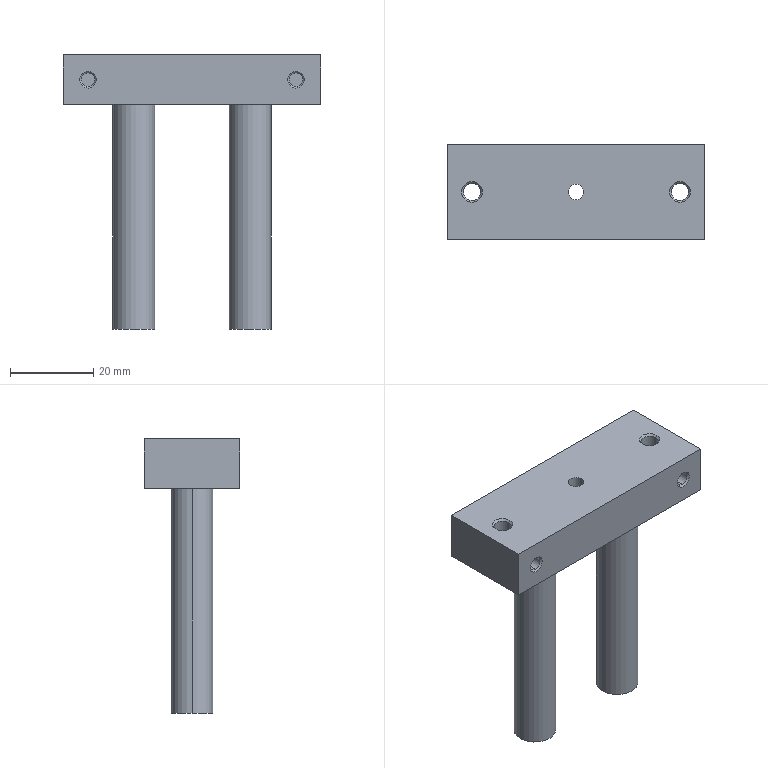Part | STEP file | rod_A_CXSM20_40_Z80_0_ | 1 solid | 42 faces | box 62 x 23 x 66 mm | volume 24938 mm3 | cylinder 18 | cone 12 | plane 12 | commonest cylinder face diameters 3.24 x8 4.13 x4 10 x4 3.732 x2
STEP:
#1=CARTESIAN_POINT('',(-1.866,12.5,12.));
#2=VERTEX_POINT('',#1);
#3=CARTESIAN_POINT('',(1.866,12.5,12.));
#4=VERTEX_POINT('',#3);
#5=CARTESIAN_POINT('',(0.,12.5,12.));
#6=DIRECTION('',(0.,0.,1.));
#7=DIRECTION('',(1.,0.,0.));
#8=AXIS2_PLACEMENT_3D('',#5,#6,#7);
#9=CIRCLE('',#8,1.866);
#10=EDGE_CURVE('',#2,#4,#9,.T.);
#11=ORIENTED_EDGE('',*,*,#10,.F.);
#12=CARTESIAN_POINT('',(-1.866,12.5,24.));
#13=VERTEX_POINT('',#12);
#14=CARTESIAN_POINT('',(-1.866,12.5,-42.));
#15=DIRECTION('',(0.,0.,1.));
#16=VECTOR('',#15,1000.);
#17=LINE('',#14,#16);
#18=EDGE_CURVE('',#2,#13,#17,.T.);
#19=ORIENTED_EDGE('',*,*,#18,.T.);
#20=CARTESIAN_POINT('',(1.866,12.5,24.));
#21=VERTEX_POINT('',#20);
#22=CARTESIAN_POINT('',(0.,12.5,24.));
#23=DIRECTION('',(0.,0.,1.));
#24=DIRECTION('',(1.,0.,0.));
#25=AXIS2_PLACEMENT_3D('',#22,#23,#24);
#26=CIRCLE('',#25,1.866);
#27=EDGE_CURVE('',#13,#21,#26,.T.);
#28=ORIENTED_EDGE('',*,*,#27,.T.);
#29=CARTESIAN_POINT('',(1.866,12.5,-42.));
#30=DIRECTION('',(0.,0.,1.));
#31=VECTOR('',#30,1000.);
#32=LINE('',#29,#31);
#33=EDGE_CURVE('',#4,#21,#32,.T.);
#34=ORIENTED_EDGE('',*,*,#33,.F.);
#35=EDGE_LOOP('',(#11,#19,#28,#34));
#36=FACE_OUTER_BOUND('',#35,.T.);
#37=CARTESIAN_POINT('',(0.,12.5,-42.));
#38=DIRECTION('',(0.,0.,1.));
#39=DIRECTION('',(1.,0.,0.));
#40=AXIS2_PLACEMENT_3D('',#37,#38,#39);
#41=CYLINDRICAL_SURFACE('',#40,1.866);
#42=ADVANCED_FACE('',(#36),#41,.F.);
#43=CARTESIAN_POINT('',(-25.,1.38,16.38));
#44=VERTEX_POINT('',#43);
#45=CARTESIAN_POINT('',(-25.,1.38,19.62));
#46=VERTEX_POINT('',#45);
#47=CARTESIAN_POINT('',(-25.,1.38,18.));
#48=DIRECTION('',(0.,1.,0.));
#49=DIRECTION('',(0.,0.,1.));
#50=AXIS2_PLACEMENT_3D('',#47,#48,#49);
#51=CIRCLE('',#50,1.62);
#52=EDGE_CURVE('',#44,#46,#51,.T.);
#53=ORIENTED_EDGE('',*,*,#52,.F.);
#54=CARTESIAN_POINT('',(-25.,7.,16.38));
#55=VERTEX_POINT('',#54);
#56=CARTESIAN_POINT('',(-25.,0.,16.38));
#57=DIRECTION('',(0.,1.,0.));
#58=VECTOR('',#57,1000.);
#59=LINE('',#56,#58);
#60=EDGE_CURVE('',#44,#55,#59,.T.);
#61=ORIENTED_EDGE('',*,*,#60,.T.);
#62=CARTESIAN_POINT('',(-25.,7.,19.62));
#63=VERTEX_POINT('',#62);
#64=CARTESIAN_POINT('',(-25.,7.,18.));
#65=DIRECTION('',(0.,1.,0.));
#66=DIRECTION('',(0.,0.,1.));
#67=AXIS2_PLACEMENT_3D('',#64,#65,#66);
#68=CIRCLE('',#67,1.62);
#69=EDGE_CURVE('',#55,#63,#68,.T.);
#70=ORIENTED_EDGE('',*,*,#69,.T.);
#71=CARTESIAN_POINT('',(-25.,0.,19.62));
#72=DIRECTION('',(0.,1.,0.));
#73=VECTOR('',#72,1000.);
#74=LINE('',#71,#73);
#75=EDGE_CURVE('',#46,#63,#74,.T.);
#76=ORIENTED_EDGE('',*,*,#75,.F.);
#77=EDGE_LOOP('',(#53,#61,#70,#76));
#78=FACE_OUTER_BOUND('',#77,.T.);
#79=CARTESIAN_POINT('',(-25.,0.,18.));
#80=DIRECTION('',(0.,1.,0.));
#81=DIRECTION('',(0.,0.,1.));
#82=AXIS2_PLACEMENT_3D('',#79,#80,#81);
#83=CYLINDRICAL_SURFACE('',#82,1.62);
#84=ADVANCED_FACE('',(#78),#83,.F.);
#85=ORIENTED_EDGE('',*,*,#52,.T.);
#86=CARTESIAN_POINT('',(-25.,1.,20.));
#87=VERTEX_POINT('',#86);
#88=CARTESIAN_POINT('',(-25.,0.,21.));
#89=DIRECTION('',(0.,-0.7071,0.7071));
#90=VECTOR('',#89,1000.);
#91=LINE('',#88,#90);
#92=EDGE_CURVE('',#46,#87,#91,.T.);
#93=ORIENTED_EDGE('',*,*,#92,.T.);
#94=CARTESIAN_POINT('',(-25.,1.,16.));
#95=VERTEX_POINT('',#94);
#96=CARTESIAN_POINT('',(-25.,1.,18.));
#97=DIRECTION('',(0.,-1.,0.));
#98=DIRECTION('',(0.,0.,1.));
#99=AXIS2_PLACEMENT_3D('',#96,#97,#98);
#100=CIRCLE('',#99,2.);
#101=EDGE_CURVE('',#87,#95,#100,.T.);
#102=ORIENTED_EDGE('',*,*,#101,.T.);
#103=CARTESIAN_POINT('',(-25.,0.,15.));
#104=DIRECTION('',(0.,-0.7071,-0.7071));
#105=VECTOR('',#104,1000.);
#106=LINE('',#103,#105);
#107=EDGE_CURVE('',#44,#95,#106,.T.);
#108=ORIENTED_EDGE('',*,*,#107,.F.);
#109=EDGE_LOOP('',(#85,#93,#102,#108));
#110=FACE_OUTER_BOUND('',#109,.T.);
#111=CARTESIAN_POINT('',(-25.,0.,18.));
#112=DIRECTION('',(0.,-1.,0.));
#113=DIRECTION('',(0.,0.,-1.));
#114=AXIS2_PLACEMENT_3D('',#111,#112,#113);
#115=CONICAL_SURFACE('',#114,3.,0.7854);
#116=ADVANCED_FACE('',(#110),#115,.F.);
#117=CARTESIAN_POINT('',(25.,1.38,16.38));
#118=VERTEX_POINT('',#117);
#119=CARTESIAN_POINT('',(25.,1.38,19.62));
#120=VERTEX_POINT('',#119);
#121=CARTESIAN_POINT('',(25.,1.38,18.));
#122=DIRECTION('',(0.,1.,0.));
#123=DIRECTION('',(0.,0.,1.));
#124=AXIS2_PLACEMENT_3D('',#121,#122,#123);
#125=CIRCLE('',#124,1.62);
#126=EDGE_CURVE('',#118,#120,#125,.T.);
#127=ORIENTED_EDGE('',*,*,#126,.F.);
#128=CARTESIAN_POINT('',(25.,7.,16.38));
#129=VERTEX_POINT('',#128);
#130=CARTESIAN_POINT('',(25.,0.,16.38));
#131=DIRECTION('',(0.,1.,0.));
#132=VECTOR('',#131,1000.);
#133=LINE('',#130,#132);
#134=EDGE_CURVE('',#118,#129,#133,.T.);
#135=ORIENTED_EDGE('',*,*,#134,.T.);
#136=CARTESIAN_POINT('',(25.,7.,19.62));
#137=VERTEX_POINT('',#136);
#138=CARTESIAN_POINT('',(25.,7.,18.));
#139=DIRECTION('',(0.,1.,0.));
#140=DIRECTION('',(0.,0.,1.));
#141=AXIS2_PLACEMENT_3D('',#138,#139,#140);
#142=CIRCLE('',#141,1.62);
#143=EDGE_CURVE('',#129,#137,#142,.T.);
#144=ORIENTED_EDGE('',*,*,#143,.T.);
#145=CARTESIAN_POINT('',(25.,0.,19.62));
#146=DIRECTION('',(0.,1.,0.));
#147=VECTOR('',#146,1000.);
#148=LINE('',#145,#147);
#149=EDGE_CURVE('',#120,#137,#148,.T.);
#150=ORIENTED_EDGE('',*,*,#149,.F.);
#151=EDGE_LOOP('',(#127,#135,#144,#150));
#152=FACE_OUTER_BOUND('',#151,.T.);
#153=CARTESIAN_POINT('',(25.,0.,18.));
#154=DIRECTION('',(0.,1.,0.));
#155=DIRECTION('',(0.,0.,1.));
#156=AXIS2_PLACEMENT_3D('',#153,#154,#155);
#157=CYLINDRICAL_SURFACE('',#156,1.62);
#158=ADVANCED_FACE('',(#152),#157,.F.);
#159=ORIENTED_EDGE('',*,*,#126,.T.);
#160=CARTESIAN_POINT('',(25.,1.,20.));
#161=VERTEX_POINT('',#160);
#162=CARTESIAN_POINT('',(25.,0.,21.));
#163=DIRECTION('',(0.,-0.7071,0.7071));
#164=VECTOR('',#163,1000.);
#165=LINE('',#162,#164);
#166=EDGE_CURVE('',#120,#161,#165,.T.);
#167=ORIENTED_EDGE('',*,*,#166,.T.);
#168=CARTESIAN_POINT('',(25.,1.,16.));
#169=VERTEX_POINT('',#168);
#170=CARTESIAN_POINT('',(25.,1.,18.));
#171=DIRECTION('',(0.,-1.,0.));
#172=DIRECTION('',(0.,0.,1.));
#173=AXIS2_PLACEMENT_3D('',#170,#171,#172);
#174=CIRCLE('',#173,2.);
#175=EDGE_CURVE('',#161,#169,#174,.T.);
#176=ORIENTED_EDGE('',*,*,#175,.T.);
#177=CARTESIAN_POINT('',(25.,0.,15.));
#178=DIRECTION('',(0.,-0.7071,-0.7071));
#179=VECTOR('',#178,1000.);
#180=LINE('',#177,#179);
#181=EDGE_CURVE('',#118,#169,#180,.T.);
#182=ORIENTED_EDGE('',*,*,#181,.F.);
#183=EDGE_LOOP('',(#159,#167,#176,#182));
#184=FACE_OUTER_BOUND('',#183,.T.);
#185=CARTESIAN_POINT('',(25.,0.,18.));
#186=DIRECTION('',(0.,-1.,0.));
#187=DIRECTION('',(0.,0.,-1.));
#188=AXIS2_PLACEMENT_3D('',#185,#186,#187);
#189=CONICAL_SURFACE('',#188,3.,0.7854);
#190=ADVANCED_FACE('',(#184),#189,.F.);
#191=CARTESIAN_POINT('',(-22.935,12.5,23.565));
#192=VERTEX_POINT('',#191);
#193=CARTESIAN_POINT('',(-27.065,12.5,23.565));
#194=VERTEX_POINT('',#193);
#195=CARTESIAN_POINT('',(-25.,12.5,23.565));
#196=DIRECTION('',(0.,0.,-1.));
#197=DIRECTION('',(-1.,0.,0.));
#198=AXIS2_PLACEMENT_3D('',#195,#196,#197);
#199=CIRCLE('',#198,2.065);
#200=EDGE_CURVE('',#192,#194,#199,.T.);
#201=ORIENTED_EDGE('',*,*,#200,.T.);
#202=CARTESIAN_POINT('',(-27.5,12.5,24.));
#203=VERTEX_POINT('',#202);
#204=CARTESIAN_POINT('',(-28.,12.5,24.5));
#205=DIRECTION('',(-0.7071,0.,0.7071));
#206=VECTOR('',#205,1000.);
#207=LINE('',#204,#206);
#208=EDGE_CURVE('',#194,#203,#207,.T.);
#209=ORIENTED_EDGE('',*,*,#208,.T.);
#210=CARTESIAN_POINT('',(-22.5,12.5,24.));
#211=VERTEX_POINT('',#210);
#212=CARTESIAN_POINT('',(-25.,12.5,24.));
#213=DIRECTION('',(0.,0.,-1.));
#214=DIRECTION('',(1.,0.,0.));
#215=AXIS2_PLACEMENT_3D('',#212,#213,#214);
#216=CIRCLE('',#215,2.5);
#217=EDGE_CURVE('',#211,#203,#216,.T.);
#218=ORIENTED_EDGE('',*,*,#217,.F.);
#219=CARTESIAN_POINT('',(-22.,12.5,24.5));
#220=DIRECTION('',(0.7071,0.,0.7071));
#221=VECTOR('',#220,1000.);
#222=LINE('',#219,#221);
#223=EDGE_CURVE('',#192,#211,#222,.T.);
#224=ORIENTED_EDGE('',*,*,#223,.F.);
#225=EDGE_LOOP('',(#201,#209,#218,#224));
#226=FACE_OUTER_BOUND('',#225,.T.);
#227=CARTESIAN_POINT('',(-25.,12.5,24.5));
#228=DIRECTION('',(0.,0.,1.));
#229=DIRECTION('',(1.,0.,0.));
#230=AXIS2_PLACEMENT_3D('',#227,#228,#229);
#231=CONICAL_SURFACE('',#230,3.,0.7854);
#232=ADVANCED_FACE('',(#226),#231,.F.);
#233=ORIENTED_EDGE('',*,*,#200,.F.);
#234=CARTESIAN_POINT('',(-22.935,12.5,12.));
#235=VERTEX_POINT('',#234);
#236=CARTESIAN_POINT('',(-22.935,12.5,24.5));
#237=DIRECTION('',(0.,0.,-1.));
#238=VECTOR('',#237,1000.);
#239=LINE('',#236,#238);
#240=EDGE_CURVE('',#192,#235,#239,.T.);
#241=ORIENTED_EDGE('',*,*,#240,.T.);
#242=CARTESIAN_POINT('',(-27.065,12.5,12.));
#243=VERTEX_POINT('',#242);
#244=CARTESIAN_POINT('',(-25.,12.5,12.));
#245=DIRECTION('',(0.,0.,-1.));
#246=DIRECTION('',(-1.,0.,0.));
#247=AXIS2_PLACEMENT_3D('',#244,#245,#246);
#248=CIRCLE('',#247,2.065);
#249=EDGE_CURVE('',#235,#243,#248,.T.);
#250=ORIENTED_EDGE('',*,*,#249,.T.);
#251=CARTESIAN_POINT('',(-27.065,12.5,24.5));
#252=DIRECTION('',(0.,0.,-1.));
#253=VECTOR('',#252,1000.);
#254=LINE('',#251,#253);
#255=EDGE_CURVE('',#194,#243,#254,.T.);
#256=ORIENTED_EDGE('',*,*,#255,.F.);
#257=EDGE_LOOP('',(#233,#241,#250,#256));
#258=FACE_OUTER_BOUND('',#257,.T.);
#259=CARTESIAN_POINT('',(-25.,12.5,24.5));
#260=DIRECTION('',(0.,0.,-1.));
#261=DIRECTION('',(-1.,0.,0.));
#262=AXIS2_PLACEMENT_3D('',#259,#260,#261);
#263=CYLINDRICAL_SURFACE('',#262,2.065);
#264=ADVANCED_FACE('',(#258),#263,.F.);
#265=CARTESIAN_POINT('',(27.065,12.5,23.565));
#266=VERTEX_POINT('',#265);
#267=CARTESIAN_POINT('',(22.935,12.5,23.565));
#268=VERTEX_POINT('',#267);
#269=CARTESIAN_POINT('',(25.,12.5,23.565));
#270=DIRECTION('',(0.,0.,-1.));
#271=DIRECTION('',(-1.,0.,0.));
#272=AXIS2_PLACEMENT_3D('',#269,#270,#271);
#273=CIRCLE('',#272,2.065);
#274=EDGE_CURVE('',#266,#268,#273,.T.);
#275=ORIENTED_EDGE('',*,*,#274,.T.);
#276=CARTESIAN_POINT('',(22.5,12.5,24.));
#277=VERTEX_POINT('',#276);
#278=CARTESIAN_POINT('',(22.,12.5,24.5));
#279=DIRECTION('',(-0.7071,0.,0.7071));
#280=VECTOR('',#279,1000.);
#281=LINE('',#278,#280);
#282=EDGE_CURVE('',#268,#277,#281,.T.);
#283=ORIENTED_EDGE('',*,*,#282,.T.);
#284=CARTESIAN_POINT('',(27.5,12.5,24.));
#285=VERTEX_POINT('',#284);
#286=CARTESIAN_POINT('',(25.,12.5,24.));
#287=DIRECTION('',(0.,0.,-1.));
#288=DIRECTION('',(1.,0.,0.));
#289=AXIS2_PLACEMENT_3D('',#286,#287,#288);
#290=CIRCLE('',#289,2.5);
#291=EDGE_CURVE('',#285,#277,#290,.T.);
#292=ORIENTED_EDGE('',*,*,#291,.F.);
#293=CARTESIAN_POINT('',(28.,12.5,24.5));
#294=DIRECTION('',(0.7071,0.,0.7071));
#295=VECTOR('',#294,1000.);
#296=LINE('',#293,#295);
#297=EDGE_CURVE('',#266,#285,#296,.T.);
#298=ORIENTED_EDGE('',*,*,#297,.F.);
#299=EDGE_LOOP('',(#275,#283,#292,#298));
#300=FACE_OUTER_BOUND('',#299,.T.);
#301=CARTESIAN_POINT('',(25.,12.5,24.5));
#302=DIRECTION('',(0.,0.,1.));
#303=DIRECTION('',(1.,0.,0.));
#304=AXIS2_PLACEMENT_3D('',#301,#302,#303);
#305=CONICAL_SURFACE('',#304,3.,0.7854);
#306=ADVANCED_FACE('',(#300),#305,.F.);
#307=ORIENTED_EDGE('',*,*,#274,.F.);
#308=CARTESIAN_POINT('',(27.065,12.5,12.));
#309=VERTEX_POINT('',#308);
#310=CARTESIAN_POINT('',(27.065,12.5,24.5));
#311=DIRECTION('',(0.,0.,-1.));
#312=VECTOR('',#311,1000.);
#313=LINE('',#310,#312);
#314=EDGE_CURVE('',#266,#309,#313,.T.);
#315=ORIENTED_EDGE('',*,*,#314,.T.);
#316=CARTESIAN_POINT('',(22.935,12.5,12.));
#317=VERTEX_POINT('',#316);
#318=CARTESIAN_POINT('',(25.,12.5,12.));
#319=DIRECTION('',(0.,0.,-1.));
#320=DIRECTION('',(-1.,0.,0.));
#321=AXIS2_PLACEMENT_3D('',#318,#319,#320);
#322=CIRCLE('',#321,2.065);
#323=EDGE_CURVE('',#309,#317,#322,.T.);
#324=ORIENTED_EDGE('',*,*,#323,.T.);
#325=CARTESIAN_POINT('',(22.935,12.5,24.5));
#326=DIRECTION('',(0.,0.,-1.));
#327=VECTOR('',#326,1000.);
#328=LINE('',#325,#327);
#329=EDGE_CURVE('',#268,#317,#328,.T.);
#330=ORIENTED_EDGE('',*,*,#329,.F.);
#331=EDGE_LOOP('',(#307,#315,#324,#330));
#332=FACE_OUTER_BOUND('',#331,.T.);
#333=CARTESIAN_POINT('',(25.,12.5,24.5));
#334=DIRECTION('',(0.,0.,-1.));
#335=DIRECTION('',(-1.,0.,0.));
#336=AXIS2_PLACEMENT_3D('',#333,#334,#335);
#337=CYLINDRICAL_SURFACE('',#336,2.065);
#338=ADVANCED_FACE('',(#332),#337,.F.);
#339=CARTESIAN_POINT('',(25.,23.62,19.62));
#340=VERTEX_POINT('',#339);
#341=CARTESIAN_POINT('',(25.,23.62,16.38));
#342=VERTEX_POINT('',#341);
#343=CARTESIAN_POINT('',(25.,23.62,18.));
#344=DIRECTION('',(0.,-1.,0.));
#345=DIRECTION('',(0.,0.,-1.));
#346=AXIS2_PLACEMENT_3D('',#343,#344,#345);
#347=CIRCLE('',#346,1.62);
#348=EDGE_CURVE('',#340,#342,#347,.T.);
#349=ORIENTED_EDGE('',*,*,#348,.F.);
#350=CARTESIAN_POINT('',(25.,18.,19.62));
#351=VERTEX_POINT('',#350);
#352=CARTESIAN_POINT('',(25.,24.5,19.62));
#353=DIRECTION('',(0.,-1.,0.));
#354=VECTOR('',#353,1000.);
#355=LINE('',#352,#354);
#356=EDGE_CURVE('',#340,#351,#355,.T.);
#357=ORIENTED_EDGE('',*,*,#356,.T.);
#358=CARTESIAN_POINT('',(25.,18.,16.38));
#359=VERTEX_POINT('',#358);
#360=CARTESIAN_POINT('',(25.,18.,18.));
#361=DIRECTION('',(0.,-1.,0.));
#362=DIRECTION('',(0.,0.,-1.));
#363=AXIS2_PLACEMENT_3D('',#360,#361,#362);
#364=CIRCLE('',#363,1.62);
#365=EDGE_CURVE('',#351,#359,#364,.T.);
#366=ORIENTED_EDGE('',*,*,#365,.T.);
#367=CARTESIAN_POINT('',(25.,24.5,16.38));
#368=DIRECTION('',(0.,-1.,0.));
#369=VECTOR('',#368,1000.);
#370=LINE('',#367,#369);
#371=EDGE_CURVE('',#342,#359,#370,.T.);
#372=ORIENTED_EDGE('',*,*,#371,.F.);
#373=EDGE_LOOP('',(#349,#357,#366,#372));
#374=FACE_OUTER_BOUND('',#373,.T.);
#375=CARTESIAN_POINT('',(25.,24.5,18.));
#376=DIRECTION('',(0.,-1.,0.));
#377=DIRECTION('',(0.,0.,-1.));
#378=AXIS2_PLACEMENT_3D('',#375,#376,#377);
#379=CYLINDRICAL_SURFACE('',#378,1.62);
#380=ADVANCED_FACE('',(#374),#379,.F.);
#381=ORIENTED_EDGE('',*,*,#348,.T.);
#382=CARTESIAN_POINT('',(25.,24.,16.));
#383=VERTEX_POINT('',#382);
#384=CARTESIAN_POINT('',(25.,24.5,15.5));
#385=DIRECTION('',(0.,0.7071,-0.7071));
#386=VECTOR('',#385,1000.);
#387=LINE('',#384,#386);
#388=EDGE_CURVE('',#342,#383,#387,.T.);
#389=ORIENTED_EDGE('',*,*,#388,.T.);
#390=CARTESIAN_POINT('',(25.,24.,20.));
#391=VERTEX_POINT('',#390);
#392=CARTESIAN_POINT('',(25.,24.,18.));
#393=DIRECTION('',(0.,1.,0.));
#394=DIRECTION('',(0.,0.,-1.));
#395=AXIS2_PLACEMENT_3D('',#392,#393,#394);
#396=CIRCLE('',#395,2.);
#397=EDGE_CURVE('',#383,#391,#396,.T.);
#398=ORIENTED_EDGE('',*,*,#397,.T.);
#399=CARTESIAN_POINT('',(25.,24.5,20.5));
#400=DIRECTION('',(0.,0.7071,0.7071));
#401=VECTOR('',#400,1000.);
#402=LINE('',#399,#401);
#403=EDGE_CURVE('',#340,#391,#402,.T.);
#404=ORIENTED_EDGE('',*,*,#403,.F.);
#405=EDGE_LOOP('',(#381,#389,#398,#404));
#406=FACE_OUTER_BOUND('',#405,.T.);
#407=CARTESIAN_POINT('',(25.,24.5,18.));
#408=DIRECTION('',(0.,1.,0.));
#409=DIRECTION('',(0.,0.,1.));
#410=AXIS2_PLACEMENT_3D('',#407,#408,#409);
#411=CONICAL_SURFACE('',#410,2.5,0.7854);
#412=ADVANCED_FACE('',(#406),#411,.F.);
#413=CARTESIAN_POINT('',(-25.,23.62,19.62));
#414=VERTEX_POINT('',#413);
#415=CARTESIAN_POINT('',(-25.,23.62,16.38));
#416=VERTEX_POINT('',#415);
#417=CARTESIAN_POINT('',(-25.,23.62,18.));
#418=DIRECTION('',(0.,-1.,0.));
#419=DIRECTION('',(0.,0.,-1.));
#420=AXIS2_PLACEMENT_3D('',#417,#418,#419);
#421=CIRCLE('',#420,1.62);
#422=EDGE_CURVE('',#414,#416,#421,.T.);
#423=ORIENTED_EDGE('',*,*,#422,.F.);
#424=CARTESIAN_POINT('',(-25.,18.,19.62));
#425=VERTEX_POINT('',#424);
#426=CARTESIAN_POINT('',(-25.,24.5,19.62));
#427=DIRECTION('',(0.,-1.,0.));
#428=VECTOR('',#427,1000.);
#429=LINE('',#426,#428);
#430=EDGE_CURVE('',#414,#425,#429,.T.);
#431=ORIENTED_EDGE('',*,*,#430,.T.);
#432=CARTESIAN_POINT('',(-25.,18.,16.38));
#433=VERTEX_POINT('',#432);
#434=CARTESIAN_POINT('',(-25.,18.,18.));
#435=DIRECTION('',(0.,-1.,0.));
#436=DIRECTION('',(0.,0.,-1.));
#437=AXIS2_PLACEMENT_3D('',#434,#435,#436);
#438=CIRCLE('',#437,1.62);
#439=EDGE_CURVE('',#425,#433,#438,.T.);
#440=ORIENTED_EDGE('',*,*,#439,.T.);
#441=CARTESIAN_POINT('',(-25.,24.5,16.38));
#442=DIRECTION('',(0.,-1.,0.));
#443=VECTOR('',#442,1000.);
#444=LINE('',#441,#443);
#445=EDGE_CURVE('',#416,#433,#444,.T.);
#446=ORIENTED_EDGE('',*,*,#445,.F.);
#447=EDGE_LOOP('',(#423,#431,#440,#446));
#448=FACE_OUTER_BOUND('',#447,.T.);
#449=CARTESIAN_POINT('',(-25.,24.5,18.));
#450=DIRECTION('',(0.,-1.,0.));
#451=DIRECTION('',(0.,0.,-1.));
#452=AXIS2_PLACEMENT_3D('',#449,#450,#451);
#453=CYLINDRICAL_SURFACE('',#452,1.62);
#454=ADVANCED_FACE('',(#448),#453,.F.);
#455=ORIENTED_EDGE('',*,*,#422,.T.);
#456=CARTESIAN_POINT('',(-25.,24.,16.));
#457=VERTEX_POINT('',#456);
#458=CARTESIAN_POINT('',(-25.,24.5,15.5));
#459=DIRECTION('',(0.,0.7071,-0.7071));
#460=VECTOR('',#459,1000.);
#461=LINE('',#458,#460);
#462=EDGE_CURVE('',#416,#457,#461,.T.);
#463=ORIENTED_EDGE('',*,*,#462,.T.);
#464=CARTESIAN_POINT('',(-25.,24.,20.));
#465=VERTEX_POINT('',#464);
#466=CARTESIAN_POINT('',(-25.,24.,18.));
#467=DIRECTION('',(0.,1.,0.));
#468=DIRECTION('',(0.,0.,-1.));
#469=AXIS2_PLACEMENT_3D('',#466,#467,#468);
#470=CIRCLE('',#469,2.);
#471=EDGE_CURVE('',#457,#465,#470,.T.);
#472=ORIENTED_EDGE('',*,*,#471,.T.);
#473=CARTESIAN_POINT('',(-25.,24.5,20.5));
#474=DIRECTION('',(0.,0.7071,0.7071));
#475=VECTOR('',#474,1000.);
#476=LINE('',#473,#475);
#477=EDGE_CURVE('',#414,#465,#476,.T.);
#478=ORIENTED_EDGE('',*,*,#477,.F.);
#479=EDGE_LOOP('',(#455,#463,#472,#478));
#480=FACE_OUTER_BOUND('',#479,.T.);
#481=CARTESIAN_POINT('',(-25.,24.5,18.));
#482=DIRECTION('',(0.,1.,0.));
#483=DIRECTION('',(0.,0.,1.));
#484=AXIS2_PLACEMENT_3D('',#481,#482,#483);
#485=CONICAL_SURFACE('',#484,2.5,0.7854);
#486=ADVANCED_FACE('',(#480),#485,.F.);
#487=CARTESIAN_POINT('',(-9.,12.5,-42.));
#488=VERTEX_POINT('',#487);
#489=CARTESIAN_POINT('',(-19.,12.5,-42.));
#490=VERTEX_POINT('',#489);
#491=CARTESIAN_POINT('',(-14.,12.5,-42.));
#492=DIRECTION('',(0.,0.,1.));
#493=DIRECTION('',(1.,0.,0.));
#494=AXIS2_PLACEMENT_3D('',#491,#492,#493);
#495=CIRCLE('',#494,5.);
#496=EDGE_CURVE('',#488,#490,#495,.T.);
#497=ORIENTED_EDGE('',*,*,#496,.T.);
#498=CARTESIAN_POINT('',(-19.,12.5,12.));
#499=VERTEX_POINT('',#498);
#500=CARTESIAN_POINT('',(-19.,12.5,-42.));
#501=DIRECTION('',(0.,0.,1.));
#502=VECTOR('',#501,1000.);
#503=LINE('',#500,#502);
#504=EDGE_CURVE('',#490,#499,#503,.T.);
#505=ORIENTED_EDGE('',*,*,#504,.T.);
#506=CARTESIAN_POINT('',(-9.,12.5,12.));
#507=VERTEX_POINT('',#506);
#508=CARTESIAN_POINT('',(-14.,12.5,12.));
#509=DIRECTION('',(0.,0.,1.));
#510=DIRECTION('',(1.,0.,0.));
#511=AXIS2_PLACEMENT_3D('',#508,#509,#510);
#512=CIRCLE('',#511,5.);
#513=EDGE_CURVE('',#507,#499,#512,.T.);
#514=ORIENTED_EDGE('',*,*,#513,.F.);
#515=CARTESIAN_POINT('',(-9.,12.5,-42.));
#516=DIRECTION('',(0.,0.,1.));
#517=VECTOR('',#516,1000.);
#518=LINE('',#515,#517);
#519=EDGE_CURVE('',#488,#507,#518,.T.);
#520=ORIENTED_EDGE('',*,*,#519,.F.);
#521=EDGE_LOOP('',(#497,#505,#514,#520));
#522=FACE_OUTER_BOUND('',#521,.T.);
#523=CARTESIAN_POINT('',(-14.,12.5,-42.));
#524=DIRECTION('',(0.,0.,1.));
#525=DIRECTION('',(1.,0.,0.));
#526=AXIS2_PLACEMENT_3D('',#523,#524,#525);
#527=CYLINDRICAL_SURFACE('',#526,5.);
#528=ADVANCED_FACE('',(#522),#527,.T.);
#529=CARTESIAN_POINT('',(19.,12.5,-42.));
#530=VERTEX_POINT('',#529);
#531=CARTESIAN_POINT('',(9.,12.5,-42.));
#532=VERTEX_POINT('',#531);
#533=CARTESIAN_POINT('',(14.,12.5,-42.));
#534=DIRECTION('',(0.,0.,1.));
#535=DIRECTION('',(1.,0.,0.));
#536=AXIS2_PLACEMENT_3D('',#533,#534,#535);
#537=CIRCLE('',#536,5.);
#538=EDGE_CURVE('',#530,#532,#537,.T.);
#539=ORIENTED_EDGE('',*,*,#538,.T.);
#540=CARTESIAN_POINT('',(9.,12.5,12.));
#541=VERTEX_POINT('',#540);
#542=CARTESIAN_POINT('',(9.,12.5,-42.));
#543=DIRECTION('',(0.,0.,1.));
#544=VECTOR('',#543,1000.);
#545=LINE('',#542,#544);
#546=EDGE_CURVE('',#532,#541,#545,.T.);
#547=ORIENTED_EDGE('',*,*,#546,.T.);
#548=CARTESIAN_POINT('',(19.,12.5,12.));
#549=VERTEX_POINT('',#548);
#550=CARTESIAN_POINT('',(14.,12.5,12.));
#551=DIRECTION('',(0.,0.,1.));
#552=DIRECTION('',(1.,0.,0.));
#553=AXIS2_PLACEMENT_3D('',#550,#551,#552);
#554=CIRCLE('',#553,5.);
#555=EDGE_CURVE('',#549,#541,#554,.T.);
#556=ORIENTED_EDGE('',*,*,#555,.F.);
#557=CARTESIAN_POINT('',(19.,12.5,-42.));
#558=DIRECTION('',(0.,0.,1.));
#559=VECTOR('',#558,1000.);
#560=LINE('',#557,#559);
#561=EDGE_CURVE('',#530,#549,#560,.T.);
#562=ORIENTED_EDGE('',*,*,#561,.F.);
#563=EDGE_LOOP('',(#539,#547,#556,#562));
#564=FACE_OUTER_BOUND('',#563,.T.);
#565=CARTESIAN_POINT('',(14.,12.5,-42.));
#566=DIRECTION('',(0.,0.,1.));
#567=DIRECTION('',(1.,0.,0.));
#568=AXIS2_PLACEMENT_3D('',#565,#566,#567);
#569=CYLINDRICAL_SURFACE('',#568,5.);
#570=ADVANCED_FACE('',(#564),#569,.T.);
#571=CARTESIAN_POINT('',(25.,1.,18.));
#572=DIRECTION('',(0.,-1.,0.));
#573=DIRECTION('',(0.,0.,1.));
#574=AXIS2_PLACEMENT_3D('',#571,#572,#573);
#575=CIRCLE('',#574,2.);
#576=EDGE_CURVE('',#169,#161,#575,.T.);
#577=ORIENTED_EDGE('',*,*,#576,.F.);
#578=ORIENTED_EDGE('',*,*,#175,.F.);
#579=EDGE_LOOP('',(#577,#578));
#580=FACE_BOUND('',#579,.T.);
#581=CARTESIAN_POINT('',(-31.,1.,12.));
#582=VERTEX_POINT('',#581);
#583=CARTESIAN_POINT('',(31.,1.,12.));
#584=VERTEX_POINT('',#583);
#585=CARTESIAN_POINT('',(-31.,1.,12.));
#586=DIRECTION('',(1.,0.,0.));
#587=VECTOR('',#586,1000.);
#588=LINE('',#585,#587);
#589=EDGE_CURVE('',#582,#584,#588,.T.);
#590=ORIENTED_EDGE('',*,*,#589,.T.);
#591=CARTESIAN_POINT('',(31.,1.,24.));
#592=VERTEX_POINT('',#591);
#593=CARTESIAN_POINT('',(31.,1.,24.));
#594=DIRECTION('',(0.,0.,-1.));
#595=VECTOR('',#594,1000.);
#596=LINE('',#593,#595);
#597=EDGE_CURVE('',#592,#584,#596,.T.);
#598=ORIENTED_EDGE('',*,*,#597,.F.);
#599=CARTESIAN_POINT('',(-31.,1.,24.));
#600=VERTEX_POINT('',#599);
#601=CARTESIAN_POINT('',(-31.,1.,24.));
#602=DIRECTION('',(1.,0.,0.));
#603=VECTOR('',#602,1000.);
#604=LINE('',#601,#603);
#605=EDGE_CURVE('',#600,#592,#604,.T.);
#606=ORIENTED_EDGE('',*,*,#605,.F.);
#607=CARTESIAN_POINT('',(-31.,1.,24.));
#608=DIRECTION('',(0.,0.,-1.));
#609=VECTOR('',#608,1000.);
#610=LINE('',#607,#609);
#611=EDGE_CURVE('',#600,#582,#610,.T.);
#612=ORIENTED_EDGE('',*,*,#611,.T.);
#613=EDGE_LOOP('',(#590,#598,#606,#612));
#614=FACE_OUTER_BOUND('',#613,.T.);
#615=CARTESIAN_POINT('',(-25.,1.,18.));
#616=DIRECTION('',(0.,-1.,0.));
#617=DIRECTION('',(0.,0.,1.));
#618=AXIS2_PLACEMENT_3D('',#615,#616,#617);
#619=CIRCLE('',#618,2.);
#620=EDGE_CURVE('',#95,#87,#619,.T.);
#621=ORIENTED_EDGE('',*,*,#620,.F.);
#622=ORIENTED_EDGE('',*,*,#101,.F.);
#623=EDGE_LOOP('',(#621,#622));
#624=FACE_BOUND('',#623,.T.);
#625=CARTESIAN_POINT('',(-31.,1.,24.));
#626=DIRECTION('',(0.,1.,0.));
#627=DIRECTION('',(0.,0.,1.));
#628=AXIS2_PLACEMENT_3D('',#625,#626,#627);
#629=PLANE('',#628);
#630=ADVANCED_FACE('',(#580,#614,#624),#629,.F.);
#631=CARTESIAN_POINT('',(0.,12.5,24.));
#632=DIRECTION('',(0.,0.,1.));
#633=DIRECTION('',(1.,0.,0.));
#634=AXIS2_PLACEMENT_3D('',#631,#632,#633);
#635=CIRCLE('',#634,1.866);
#636=EDGE_CURVE('',#21,#13,#635,.T.);
#637=ORIENTED_EDGE('',*,*,#636,.F.);
#638=ORIENTED_EDGE('',*,*,#27,.F.);
#639=EDGE_LOOP('',(#637,#638));
#640=FACE_BOUND('',#639,.T.);
#641=ORIENTED_EDGE('',*,*,#291,.T.);
#642=CARTESIAN_POINT('',(25.,12.5,24.));
#643=DIRECTION('',(0.,0.,-1.));
#644=DIRECTION('',(1.,0.,0.));
#645=AXIS2_PLACEMENT_3D('',#642,#643,#644);
#646=CIRCLE('',#645,2.5);
#647=EDGE_CURVE('',#277,#285,#646,.T.);
#648=ORIENTED_EDGE('',*,*,#647,.T.);
#649=EDGE_LOOP('',(#641,#648));
#650=FACE_BOUND('',#649,.T.);
#651=CARTESIAN_POINT('',(-31.,24.,24.));
#652=VERTEX_POINT('',#651);
#653=CARTESIAN_POINT('',(-31.,24.,24.));
#654=DIRECTION('',(0.,-1.,0.));
#655=VECTOR('',#654,1000.);
#656=LINE('',#653,#655);
#657=EDGE_CURVE('',#652,#600,#656,.T.);
#658=ORIENTED_EDGE('',*,*,#657,.T.);
#659=ORIENTED_EDGE('',*,*,#605,.T.);
#660=CARTESIAN_POINT('',(31.,24.,24.));
#661=VERTEX_POINT('',#660);
#662=CARTESIAN_POINT('',(31.,1.,24.));
#663=DIRECTION('',(0.,1.,0.));
#664=VECTOR('',#663,1000.);
#665=LINE('',#662,#664);
#666=EDGE_CURVE('',#592,#661,#665,.T.);
#667=ORIENTED_EDGE('',*,*,#666,.T.);
#668=CARTESIAN_POINT('',(31.,24.,24.));
#669=DIRECTION('',(-1.,0.,0.));
#670=VECTOR('',#669,1000.);
#671=LINE('',#668,#670);
#672=EDGE_CURVE('',#661,#652,#671,.T.);
#673=ORIENTED_EDGE('',*,*,#672,.T.);
#674=EDGE_LOOP('',(#658,#659,#667,#673));
#675=FACE_OUTER_BOUND('',#674,.T.);
#676=ORIENTED_EDGE('',*,*,#217,.T.);
#677=CARTESIAN_POINT('',(-25.,12.5,24.));
#678=DIRECTION('',(0.,0.,-1.));
#679=DIRECTION('',(1.,0.,0.));
#680=AXIS2_PLACEMENT_3D('',#677,#678,#679);
#681=CIRCLE('',#680,2.5);
#682=EDGE_CURVE('',#203,#211,#681,.T.);
#683=ORIENTED_EDGE('',*,*,#682,.T.);
#684=EDGE_LOOP('',(#676,#683));
#685=FACE_BOUND('',#684,.T.);
#686=CARTESIAN_POINT('',(-31.,1.,24.));
#687=DIRECTION('',(0.,0.,1.));
#688=DIRECTION('',(1.,0.,0.));
#689=AXIS2_PLACEMENT_3D('',#686,#687,#688);
#690=PLANE('',#689);
#691=ADVANCED_FACE('',(#640,#650,#675,#685),#690,.T.);
#692=CARTESIAN_POINT('',(0.,12.5,12.));
#693=DIRECTION('',(0.,0.,1.));
#694=DIRECTION('',(1.,0.,0.));
#695=AXIS2_PLACEMENT_3D('',#692,#693,#694);
#696=CIRCLE('',#695,1.866);
#697=EDGE_CURVE('',#4,#2,#696,.T.);
#698=ORIENTED_EDGE('',*,*,#697,.T.);
#699=ORIENTED_EDGE('',*,*,#10,.T.);
#700=EDGE_LOOP('',(#698,#699));
#701=FACE_BOUND('',#700,.T.);
#702=CARTESIAN_POINT('',(25.,12.5,12.));
#703=DIRECTION('',(0.,0.,-1.));
#704=DIRECTION('',(-1.,0.,0.));
#705=AXIS2_PLACEMENT_3D('',#702,#703,#704);
#706=CIRCLE('',#705,2.065);
#707=EDGE_CURVE('',#317,#309,#706,.T.);
#708=ORIENTED_EDGE('',*,*,#707,.F.);
#709=ORIENTED_EDGE('',*,*,#323,.F.);
#710=EDGE_LOOP('',(#708,#709));
#711=FACE_BOUND('',#710,.T.);
#712=ORIENTED_EDGE('',*,*,#513,.T.);
#713=CARTESIAN_POINT('',(-14.,12.5,12.));
#714=DIRECTION('',(0.,0.,1.));
#715=DIRECTION('',(1.,0.,0.));
#716=AXIS2_PLACEMENT_3D('',#713,#714,#715);
#717=CIRCLE('',#716,5.);
#718=EDGE_CURVE('',#499,#507,#717,.T.);
#719=ORIENTED_EDGE('',*,*,#718,.T.);
#720=EDGE_LOOP('',(#712,#719));
#721=FACE_BOUND('',#720,.T.);
#722=ORIENTED_EDGE('',*,*,#555,.T.);
#723=CARTESIAN_POINT('',(14.,12.5,12.));
#724=DIRECTION('',(0.,0.,1.));
#725=DIRECTION('',(1.,0.,0.));
#726=AXIS2_PLACEMENT_3D('',#723,#724,#725);
#727=CIRCLE('',#726,5.);
#728=EDGE_CURVE('',#541,#549,#727,.T.);
#729=ORIENTED_EDGE('',*,*,#728,.T.);
#730=EDGE_LOOP('',(#722,#729));
#731=FACE_BOUND('',#730,.T.);
#732=CARTESIAN_POINT('',(-31.,24.,12.));
#733=VERTEX_POINT('',#732);
#734=CARTESIAN_POINT('',(-31.,24.,12.));
#735=DIRECTION('',(0.,-1.,0.));
#736=VECTOR('',#735,1000.);
#737=LINE('',#734,#736);
#738=EDGE_CURVE('',#733,#582,#737,.T.);
#739=ORIENTED_EDGE('',*,*,#738,.F.);
#740=CARTESIAN_POINT('',(31.,24.,12.));
#741=VERTEX_POINT('',#740);
#742=CARTESIAN_POINT('',(31.,24.,12.));
#743=DIRECTION('',(-1.,0.,0.));
#744=VECTOR('',#743,1000.);
#745=LINE('',#742,#744);
#746=EDGE_CURVE('',#741,#733,#745,.T.);
#747=ORIENTED_EDGE('',*,*,#746,.F.);
#748=CARTESIAN_POINT('',(31.,1.,12.));
#749=DIRECTION('',(0.,1.,0.));
#750=VECTOR('',#749,1000.);
#751=LINE('',#748,#750);
#752=EDGE_CURVE('',#584,#741,#751,.T.);
#753=ORIENTED_EDGE('',*,*,#752,.F.);
#754=ORIENTED_EDGE('',*,*,#589,.F.);
#755=EDGE_LOOP('',(#739,#747,#753,#754));
#756=FACE_OUTER_BOUND('',#755,.T.);
#757=CARTESIAN_POINT('',(-25.,12.5,12.));
#758=DIRECTION('',(0.,0.,-1.));
#759=DIRECTION('',(-1.,0.,0.));
#760=AXIS2_PLACEMENT_3D('',#757,#758,#759);
#761=CIRCLE('',#760,2.065);
#762=EDGE_CURVE('',#243,#235,#761,.T.);
#763=ORIENTED_EDGE('',*,*,#762,.F.);
#764=ORIENTED_EDGE('',*,*,#249,.F.);
#765=EDGE_LOOP('',(#763,#764));
#766=FACE_BOUND('',#765,.T.);
#767=CARTESIAN_POINT('',(-31.,1.,12.));
#768=DIRECTION('',(0.,0.,1.));
#769=DIRECTION('',(1.,0.,0.));
#770=AXIS2_PLACEMENT_3D('',#767,#768,#769);
#771=PLANE('',#770);
#772=ADVANCED_FACE('',(#701,#711,#721,#731,#756,#766),#771,.F.);
#773=CARTESIAN_POINT('',(-25.,24.,18.));
#774=DIRECTION('',(0.,1.,0.));
#775=DIRECTION('',(0.,0.,-1.));
#776=AXIS2_PLACEMENT_3D('',#773,#774,#775);
#777=CIRCLE('',#776,2.);
#778=EDGE_CURVE('',#465,#457,#777,.T.);
#779=ORIENTED_EDGE('',*,*,#778,.F.);
#780=ORIENTED_EDGE('',*,*,#471,.F.);
#781=EDGE_LOOP('',(#779,#780));
#782=FACE_BOUND('',#781,.T.);
#783=ORIENTED_EDGE('',*,*,#746,.T.);
#784=CARTESIAN_POINT('',(-31.,24.,24.));
#785=DIRECTION('',(0.,0.,-1.));
#786=VECTOR('',#785,1000.);
#787=LINE('',#784,#786);
#788=EDGE_CURVE('',#652,#733,#787,.T.);
#789=ORIENTED_EDGE('',*,*,#788,.F.);
#790=ORIENTED_EDGE('',*,*,#672,.F.);
#791=CARTESIAN_POINT('',(31.,24.,24.));
#792=DIRECTION('',(0.,0.,-1.));
#793=VECTOR('',#792,1000.);
#794=LINE('',#791,#793);
#795=EDGE_CURVE('',#661,#741,#794,.T.);
#796=ORIENTED_EDGE('',*,*,#795,.T.);
#797=EDGE_LOOP('',(#783,#789,#790,#796));
#798=FACE_OUTER_BOUND('',#797,.T.);
#799=CARTESIAN_POINT('',(25.,24.,18.));
#800=DIRECTION('',(0.,1.,0.));
#801=DIRECTION('',(0.,0.,-1.));
#802=AXIS2_PLACEMENT_3D('',#799,#800,#801);
#803=CIRCLE('',#802,2.);
#804=EDGE_CURVE('',#391,#383,#803,.T.);
#805=ORIENTED_EDGE('',*,*,#804,.F.);
#806=ORIENTED_EDGE('',*,*,#397,.F.);
#807=EDGE_LOOP('',(#805,#806));
#808=FACE_BOUND('',#807,.T.);
#809=CARTESIAN_POINT('',(31.,24.,24.));
#810=DIRECTION('',(0.,-1.,0.));
#811=DIRECTION('',(0.,0.,-1.));
#812=AXIS2_PLACEMENT_3D('',#809,#810,#811);
#813=PLANE('',#812);
#814=ADVANCED_FACE('',(#782,#798,#808),#813,.F.);
#815=ORIENTED_EDGE('',*,*,#738,.T.);
#816=ORIENTED_EDGE('',*,*,#611,.F.);
#817=ORIENTED_EDGE('',*,*,#657,.F.);
#818=ORIENTED_EDGE('',*,*,#788,.T.);
#819=EDGE_LOOP('',(#815,#816,#817,#818));
#820=FACE_OUTER_BOUND('',#819,.T.);
#821=CARTESIAN_POINT('',(-31.,24.,24.));
#822=DIRECTION('',(1.,0.,0.));
#823=DIRECTION('',(0.,0.,-1.));
#824=AXIS2_PLACEMENT_3D('',#821,#822,#823);
#825=PLANE('',#824);
#826=ADVANCED_FACE('',(#820),#825,.F.);
#827=ORIENTED_EDGE('',*,*,#752,.T.);
#828=ORIENTED_EDGE('',*,*,#795,.F.);
#829=ORIENTED_EDGE('',*,*,#666,.F.);
#830=ORIENTED_EDGE('',*,*,#597,.T.);
#831=EDGE_LOOP('',(#827,#828,#829,#830));
#832=FACE_OUTER_BOUND('',#831,.T.);
#833=CARTESIAN_POINT('',(31.,1.,24.));
#834=DIRECTION('',(-1.,0.,0.));
#835=DIRECTION('',(0.,0.,1.));
#836=AXIS2_PLACEMENT_3D('',#833,#834,#835);
#837=PLANE('',#836);
#838=ADVANCED_FACE('',(#832),#837,.F.);
#839=ORIENTED_EDGE('',*,*,#546,.F.);
#840=CARTESIAN_POINT('',(14.,12.5,-42.));
#841=DIRECTION('',(0.,0.,1.));
#842=DIRECTION('',(1.,0.,0.));
#843=AXIS2_PLACEMENT_3D('',#840,#841,#842);
#844=CIRCLE('',#843,5.);
#845=EDGE_CURVE('',#532,#530,#844,.T.);
#846=ORIENTED_EDGE('',*,*,#845,.T.);
#847=ORIENTED_EDGE('',*,*,#561,.T.);
#848=ORIENTED_EDGE('',*,*,#728,.F.);
#849=EDGE_LOOP('',(#839,#846,#847,#848));
#850=FACE_OUTER_BOUND('',#849,.T.);
#851=CARTESIAN_POINT('',(14.,12.5,-42.));
#852=DIRECTION('',(0.,0.,1.));
#853=DIRECTION('',(1.,0.,0.));
#854=AXIS2_PLACEMENT_3D('',#851,#852,#853);
#855=CYLINDRICAL_SURFACE('',#854,5.);
#856=ADVANCED_FACE('',(#850),#855,.T.);
#857=ORIENTED_EDGE('',*,*,#538,.F.);
#858=ORIENTED_EDGE('',*,*,#845,.F.);
#859=EDGE_LOOP('',(#857,#858));
#860=FACE_OUTER_BOUND('',#859,.T.);
#861=CARTESIAN_POINT('',(14.,12.5,-42.));
#862=DIRECTION('',(0.,0.,1.));
#863=DIRECTION('',(1.,0.,0.));
#864=AXIS2_PLACEMENT_3D('',#861,#862,#863);
#865=PLANE('',#864);
#866=ADVANCED_FACE('',(#860),#865,.F.);
#867=ORIENTED_EDGE('',*,*,#504,.F.);
#868=CARTESIAN_POINT('',(-14.,12.5,-42.));
#869=DIRECTION('',(0.,0.,1.));
#870=DIRECTION('',(1.,0.,0.));
#871=AXIS2_PLACEMENT_3D('',#868,#869,#870);
#872=CIRCLE('',#871,5.);
#873=EDGE_CURVE('',#490,#488,#872,.T.);
#874=ORIENTED_EDGE('',*,*,#873,.T.);
#875=ORIENTED_EDGE('',*,*,#519,.T.);
#876=ORIENTED_EDGE('',*,*,#718,.F.);
#877=EDGE_LOOP('',(#867,#874,#875,#876));
#878=FACE_OUTER_BOUND('',#877,.T.);
#879=CARTESIAN_POINT('',(-14.,12.5,-42.));
#880=DIRECTION('',(0.,0.,1.));
#881=DIRECTION('',(1.,0.,0.));
#882=AXIS2_PLACEMENT_3D('',#879,#880,#881);
#883=CYLINDRICAL_SURFACE('',#882,5.);
#884=ADVANCED_FACE('',(#878),#883,.T.);
#885=ORIENTED_EDGE('',*,*,#496,.F.);
#886=ORIENTED_EDGE('',*,*,#873,.F.);
#887=EDGE_LOOP('',(#885,#886));
#888=FACE_OUTER_BOUND('',#887,.T.);
#889=CARTESIAN_POINT('',(-14.,12.5,-42.));
#890=DIRECTION('',(0.,0.,1.));
#891=DIRECTION('',(1.,0.,0.));
#892=AXIS2_PLACEMENT_3D('',#889,#890,#891);
#893=PLANE('',#892);
#894=ADVANCED_FACE('',(#888),#893,.F.);
#895=ORIENTED_EDGE('',*,*,#462,.F.);
#896=CARTESIAN_POINT('',(-25.,23.62,18.));
#897=DIRECTION('',(0.,-1.,0.));
#898=DIRECTION('',(0.,0.,-1.));
#899=AXIS2_PLACEMENT_3D('',#896,#897,#898);
#900=CIRCLE('',#899,1.62);
#901=EDGE_CURVE('',#416,#414,#900,.T.);
#902=ORIENTED_EDGE('',*,*,#901,.T.);
#903=ORIENTED_EDGE('',*,*,#477,.T.);
#904=ORIENTED_EDGE('',*,*,#778,.T.);
#905=EDGE_LOOP('',(#895,#902,#903,#904));
#906=FACE_OUTER_BOUND('',#905,.T.);
#907=CARTESIAN_POINT('',(-25.,24.5,18.));
#908=DIRECTION('',(0.,1.,0.));
#909=DIRECTION('',(0.,0.,1.));
#910=AXIS2_PLACEMENT_3D('',#907,#908,#909);
#911=CONICAL_SURFACE('',#910,2.5,0.7854);
#912=ADVANCED_FACE('',(#906),#911,.F.);
#913=CARTESIAN_POINT('',(-25.,18.,18.));
#914=DIRECTION('',(0.,-1.,0.));
#915=DIRECTION('',(0.,0.,-1.));
#916=AXIS2_PLACEMENT_3D('',#913,#914,#915);
#917=CIRCLE('',#916,1.62);
#918=EDGE_CURVE('',#433,#425,#917,.T.);
#919=ORIENTED_EDGE('',*,*,#918,.F.);
#920=ORIENTED_EDGE('',*,*,#439,.F.);
#921=EDGE_LOOP('',(#919,#920));
#922=FACE_OUTER_BOUND('',#921,.T.);
#923=CARTESIAN_POINT('',(-25.,18.,18.));
#924=DIRECTION('',(0.,1.,0.));
#925=DIRECTION('',(0.,0.,1.));
#926=AXIS2_PLACEMENT_3D('',#923,#924,#925);
#927=PLANE('',#926);
#928=ADVANCED_FACE('',(#922),#927,.T.);
#929=ORIENTED_EDGE('',*,*,#430,.F.);
#930=ORIENTED_EDGE('',*,*,#901,.F.);
#931=ORIENTED_EDGE('',*,*,#445,.T.);
#932=ORIENTED_EDGE('',*,*,#918,.T.);
#933=EDGE_LOOP('',(#929,#930,#931,#932));
#934=FACE_OUTER_BOUND('',#933,.T.);
#935=CARTESIAN_POINT('',(-25.,24.5,18.));
#936=DIRECTION('',(0.,-1.,0.));
#937=DIRECTION('',(0.,0.,-1.));
#938=AXIS2_PLACEMENT_3D('',#935,#936,#937);
#939=CYLINDRICAL_SURFACE('',#938,1.62);
#940=ADVANCED_FACE('',(#934),#939,.F.);
#941=ORIENTED_EDGE('',*,*,#388,.F.);
#942=CARTESIAN_POINT('',(25.,23.62,18.));
#943=DIRECTION('',(0.,-1.,0.));
#944=DIRECTION('',(0.,0.,-1.));
#945=AXIS2_PLACEMENT_3D('',#942,#943,#944);
#946=CIRCLE('',#945,1.62);
#947=EDGE_CURVE('',#342,#340,#946,.T.);
#948=ORIENTED_EDGE('',*,*,#947,.T.);
#949=ORIENTED_EDGE('',*,*,#403,.T.);
#950=ORIENTED_EDGE('',*,*,#804,.T.);
#951=EDGE_LOOP('',(#941,#948,#949,#950));
#952=FACE_OUTER_BOUND('',#951,.T.);
#953=CARTESIAN_POINT('',(25.,24.5,18.));
#954=DIRECTION('',(0.,1.,0.));
#955=DIRECTION('',(0.,0.,1.));
#956=AXIS2_PLACEMENT_3D('',#953,#954,#955);
#957=CONICAL_SURFACE('',#956,2.5,0.7854);
#958=ADVANCED_FACE('',(#952),#957,.F.);
#959=CARTESIAN_POINT('',(25.,18.,18.));
#960=DIRECTION('',(0.,-1.,0.));
#961=DIRECTION('',(0.,0.,-1.));
#962=AXIS2_PLACEMENT_3D('',#959,#960,#961);
#963=CIRCLE('',#962,1.62);
#964=EDGE_CURVE('',#359,#351,#963,.T.);
#965=ORIENTED_EDGE('',*,*,#964,.F.);
#966=ORIENTED_EDGE('',*,*,#365,.F.);
#967=EDGE_LOOP('',(#965,#966));
#968=FACE_OUTER_BOUND('',#967,.T.);
#969=CARTESIAN_POINT('',(25.,18.,18.));
#970=DIRECTION('',(0.,1.,0.));
#971=DIRECTION('',(0.,0.,1.));
#972=AXIS2_PLACEMENT_3D('',#969,#970,#971);
#973=PLANE('',#972);
#974=ADVANCED_FACE('',(#968),#973,.T.);
#975=ORIENTED_EDGE('',*,*,#356,.F.);
#976=ORIENTED_EDGE('',*,*,#947,.F.);
#977=ORIENTED_EDGE('',*,*,#371,.T.);
#978=ORIENTED_EDGE('',*,*,#964,.T.);
#979=EDGE_LOOP('',(#975,#976,#977,#978));
#980=FACE_OUTER_BOUND('',#979,.T.);
#981=CARTESIAN_POINT('',(25.,24.5,18.));
#982=DIRECTION('',(0.,-1.,0.));
#983=DIRECTION('',(0.,0.,-1.));
#984=AXIS2_PLACEMENT_3D('',#981,#982,#983);
#985=CYLINDRICAL_SURFACE('',#984,1.62);
#986=ADVANCED_FACE('',(#980),#985,.F.);
#987=ORIENTED_EDGE('',*,*,#314,.F.);
#988=CARTESIAN_POINT('',(25.,12.5,23.565));
#989=DIRECTION('',(0.,0.,-1.));
#990=DIRECTION('',(-1.,0.,0.));
#991=AXIS2_PLACEMENT_3D('',#988,#989,#990);
#992=CIRCLE('',#991,2.065);
#993=EDGE_CURVE('',#268,#266,#992,.T.);
#994=ORIENTED_EDGE('',*,*,#993,.F.);
#995=ORIENTED_EDGE('',*,*,#329,.T.);
#996=ORIENTED_EDGE('',*,*,#707,.T.);
#997=EDGE_LOOP('',(#987,#994,#995,#996));
#998=FACE_OUTER_BOUND('',#997,.T.);
#999=CARTESIAN_POINT('',(25.,12.5,24.5));
#1000=DIRECTION('',(0.,0.,-1.));
#1001=DIRECTION('',(-1.,0.,0.));
#1002=AXIS2_PLACEMENT_3D('',#999,#1000,#1001);
#1003=CYLINDRICAL_SURFACE('',#1002,2.065);
#1004=ADVANCED_FACE('',(#998),#1003,.F.);
#1005=ORIENTED_EDGE('',*,*,#282,.F.);
#1006=ORIENTED_EDGE('',*,*,#993,.T.);
#1007=ORIENTED_EDGE('',*,*,#297,.T.);
#1008=ORIENTED_EDGE('',*,*,#647,.F.);
#1009=EDGE_LOOP('',(#1005,#1006,#1007,#1008));
#1010=FACE_OUTER_BOUND('',#1009,.T.);
#1011=CARTESIAN_POINT('',(25.,12.5,24.5));
#1012=DIRECTION('',(0.,0.,1.));
#1013=DIRECTION('',(1.,0.,0.));
#1014=AXIS2_PLACEMENT_3D('',#1011,#1012,#1013);
#1015=CONICAL_SURFACE('',#1014,3.,0.7854);
#1016=ADVANCED_FACE('',(#1010),#1015,.F.);
#1017=ORIENTED_EDGE('',*,*,#240,.F.);
#1018=CARTESIAN_POINT('',(-25.,12.5,23.565));
#1019=DIRECTION('',(0.,0.,-1.));
#1020=DIRECTION('',(-1.,0.,0.));
#1021=AXIS2_PLACEMENT_3D('',#1018,#1019,#1020);
#1022=CIRCLE('',#1021,2.065);
#1023=EDGE_CURVE('',#194,#192,#1022,.T.);
#1024=ORIENTED_EDGE('',*,*,#1023,.F.);
#1025=ORIENTED_EDGE('',*,*,#255,.T.);
#1026=ORIENTED_EDGE('',*,*,#762,.T.);
#1027=EDGE_LOOP('',(#1017,#1024,#1025,#1026));
#1028=FACE_OUTER_BOUND('',#1027,.T.);
#1029=CARTESIAN_POINT('',(-25.,12.5,24.5));
#1030=DIRECTION('',(0.,0.,-1.));
#1031=DIRECTION('',(-1.,0.,0.));
#1032=AXIS2_PLACEMENT_3D('',#1029,#1030,#1031);
#1033=CYLINDRICAL_SURFACE('',#1032,2.065);
#1034=ADVANCED_FACE('',(#1028),#1033,.F.);
#1035=ORIENTED_EDGE('',*,*,#208,.F.);
#1036=ORIENTED_EDGE('',*,*,#1023,.T.);
#1037=ORIENTED_EDGE('',*,*,#223,.T.);
#1038=ORIENTED_EDGE('',*,*,#682,.F.);
#1039=EDGE_LOOP('',(#1035,#1036,#1037,#1038));
#1040=FACE_OUTER_BOUND('',#1039,.T.);
#1041=CARTESIAN_POINT('',(-25.,12.5,24.5));
#1042=DIRECTION('',(0.,0.,1.));
#1043=DIRECTION('',(1.,0.,0.));
#1044=AXIS2_PLACEMENT_3D('',#1041,#1042,#1043);
#1045=CONICAL_SURFACE('',#1044,3.,0.7854);
#1046=ADVANCED_FACE('',(#1040),#1045,.F.);
#1047=ORIENTED_EDGE('',*,*,#166,.F.);
#1048=CARTESIAN_POINT('',(25.,1.38,18.));
#1049=DIRECTION('',(0.,1.,0.));
#1050=DIRECTION('',(0.,0.,1.));
#1051=AXIS2_PLACEMENT_3D('',#1048,#1049,#1050);
#1052=CIRCLE('',#1051,1.62);
#1053=EDGE_CURVE('',#120,#118,#1052,.T.);
#1054=ORIENTED_EDGE('',*,*,#1053,.T.);
#1055=ORIENTED_EDGE('',*,*,#181,.T.);
#1056=ORIENTED_EDGE('',*,*,#576,.T.);
#1057=EDGE_LOOP('',(#1047,#1054,#1055,#1056));
#1058=FACE_OUTER_BOUND('',#1057,.T.);
#1059=CARTESIAN_POINT('',(25.,0.,18.));
#1060=DIRECTION('',(0.,-1.,0.));
#1061=DIRECTION('',(0.,0.,-1.));
#1062=AXIS2_PLACEMENT_3D('',#1059,#1060,#1061);
#1063=CONICAL_SURFACE('',#1062,3.,0.7854);
#1064=ADVANCED_FACE('',(#1058),#1063,.F.);
#1065=CARTESIAN_POINT('',(25.,7.,18.));
#1066=DIRECTION('',(0.,1.,0.));
#1067=DIRECTION('',(0.,0.,1.));
#1068=AXIS2_PLACEMENT_3D('',#1065,#1066,#1067);
#1069=CIRCLE('',#1068,1.62);
#1070=EDGE_CURVE('',#137,#129,#1069,.T.);
#1071=ORIENTED_EDGE('',*,*,#1070,.F.);
#1072=ORIENTED_EDGE('',*,*,#143,.F.);
#1073=EDGE_LOOP('',(#1071,#1072));
#1074=FACE_OUTER_BOUND('',#1073,.T.);
#1075=CARTESIAN_POINT('',(25.,7.,18.));
#1076=DIRECTION('',(0.,-1.,0.));
#1077=DIRECTION('',(0.,0.,-1.));
#1078=AXIS2_PLACEMENT_3D('',#1075,#1076,#1077);
#1079=PLANE('',#1078);
#1080=ADVANCED_FACE('',(#1074),#1079,.T.);
#1081=ORIENTED_EDGE('',*,*,#134,.F.);
#1082=ORIENTED_EDGE('',*,*,#1053,.F.);
#1083=ORIENTED_EDGE('',*,*,#149,.T.);
#1084=ORIENTED_EDGE('',*,*,#1070,.T.);
#1085=EDGE_LOOP('',(#1081,#1082,#1083,#1084));
#1086=FACE_OUTER_BOUND('',#1085,.T.);
#1087=CARTESIAN_POINT('',(25.,0.,18.));
#1088=DIRECTION('',(0.,1.,0.));
#1089=DIRECTION('',(0.,0.,1.));
#1090=AXIS2_PLACEMENT_3D('',#1087,#1088,#1089);
#1091=CYLINDRICAL_SURFACE('',#1090,1.62);
#1092=ADVANCED_FACE('',(#1086),#1091,.F.);
#1093=ORIENTED_EDGE('',*,*,#92,.F.);
#1094=CARTESIAN_POINT('',(-25.,1.38,18.));
#1095=DIRECTION('',(0.,1.,0.));
#1096=DIRECTION('',(0.,0.,1.));
#1097=AXIS2_PLACEMENT_3D('',#1094,#1095,#1096);
#1098=CIRCLE('',#1097,1.62);
#1099=EDGE_CURVE('',#46,#44,#1098,.T.);
#1100=ORIENTED_EDGE('',*,*,#1099,.T.);
#1101=ORIENTED_EDGE('',*,*,#107,.T.);
#1102=ORIENTED_EDGE('',*,*,#620,.T.);
#1103=EDGE_LOOP('',(#1093,#1100,#1101,#1102));
#1104=FACE_OUTER_BOUND('',#1103,.T.);
#1105=CARTESIAN_POINT('',(-25.,0.,18.));
#1106=DIRECTION('',(0.,-1.,0.));
#1107=DIRECTION('',(0.,0.,-1.));
#1108=AXIS2_PLACEMENT_3D('',#1105,#1106,#1107);
#1109=CONICAL_SURFACE('',#1108,3.,0.7854);
#1110=ADVANCED_FACE('',(#1104),#1109,.F.);
#1111=CARTESIAN_POINT('',(-25.,7.,18.));
#1112=DIRECTION('',(0.,1.,0.));
#1113=DIRECTION('',(0.,0.,1.));
#1114=AXIS2_PLACEMENT_3D('',#1111,#1112,#1113);
#1115=CIRCLE('',#1114,1.62);
#1116=EDGE_CURVE('',#63,#55,#1115,.T.);
#1117=ORIENTED_EDGE('',*,*,#1116,.F.);
#1118=ORIENTED_EDGE('',*,*,#69,.F.);
#1119=EDGE_LOOP('',(#1117,#1118));
#1120=FACE_OUTER_BOUND('',#1119,.T.);
#1121=CARTESIAN_POINT('',(-25.,7.,18.));
#1122=DIRECTION('',(0.,-1.,0.));
#1123=DIRECTION('',(0.,0.,-1.));
#1124=AXIS2_PLACEMENT_3D('',#1121,#1122,#1123);
#1125=PLANE('',#1124);
#1126=ADVANCED_FACE('',(#1120),#1125,.T.);
#1127=ORIENTED_EDGE('',*,*,#60,.F.);
#1128=ORIENTED_EDGE('',*,*,#1099,.F.);
#1129=ORIENTED_EDGE('',*,*,#75,.T.);
#1130=ORIENTED_EDGE('',*,*,#1116,.T.);
#1131=EDGE_LOOP('',(#1127,#1128,#1129,#1130));
#1132=FACE_OUTER_BOUND('',#1131,.T.);
#1133=CARTESIAN_POINT('',(-25.,0.,18.));
#1134=DIRECTION('',(0.,1.,0.));
#1135=DIRECTION('',(0.,0.,1.));
#1136=AXIS2_PLACEMENT_3D('',#1133,#1134,#1135);
#1137=CYLINDRICAL_SURFACE('',#1136,1.62);
#1138=ADVANCED_FACE('',(#1132),#1137,.F.);
#1139=ORIENTED_EDGE('',*,*,#18,.F.);
#1140=ORIENTED_EDGE('',*,*,#697,.F.);
#1141=ORIENTED_EDGE('',*,*,#33,.T.);
#1142=ORIENTED_EDGE('',*,*,#636,.T.);
#1143=EDGE_LOOP('',(#1139,#1140,#1141,#1142));
#1144=FACE_OUTER_BOUND('',#1143,.T.);
#1145=CARTESIAN_POINT('',(0.,12.5,-42.));
#1146=DIRECTION('',(0.,0.,1.));
#1147=DIRECTION('',(1.,0.,0.));
#1148=AXIS2_PLACEMENT_3D('',#1145,#1146,#1147);
#1149=CYLINDRICAL_SURFACE('',#1148,1.866);
#1150=ADVANCED_FACE('',(#1144),#1149,.F.);
#1151=CLOSED_SHELL('',(#42,#84,#116,#158,#190,#232,#264,#306,#338,#380,#412,#454,#486,#528,#570,#630,#691,#772,#814,#826,#838,#856,#866,#884,#894,#912,#928,#940,#958,#974,#986,#1004,#1016,#1034,#1046,#1064,#1080,#1092,#1110,#1126,#1138,#1150));
#1152=MANIFOLD_SOLID_BREP('',#1151);
#1153=CARTESIAN_POINT('',(0.,0.,0.));
#1154=DIRECTION('',(0.,0.,1.));
#1155=DIRECTION('',(1.,0.,0.));
#1156=AXIS2_PLACEMENT_3D('',#1153,#1154,#1155);
#1157=(LENGTH_UNIT()NAMED_UNIT(*)SI_UNIT(.MILLI.,.METRE.));
#1158=UNCERTAINTY_MEASURE_WITH_UNIT(LENGTH_MEASURE(0.00001),#1157,'','');
#1159=(NAMED_UNIT(*)PLANE_ANGLE_UNIT()SI_UNIT($,.RADIAN.));
#1160=(NAMED_UNIT(*)SI_UNIT($,.STERADIAN.)SOLID_ANGLE_UNIT());
#1161=(GEOMETRIC_REPRESENTATION_CONTEXT(3)GLOBAL_UNCERTAINTY_ASSIGNED_CONTEXT((#1158))GLOBAL_UNIT_ASSIGNED_CONTEXT((#1157,#1159,#1160))REPRESENTATION_CONTEXT('',''));
#1162=ADVANCED_BREP_SHAPE_REPRESENTATION('',(#1152,#1156),#1161);